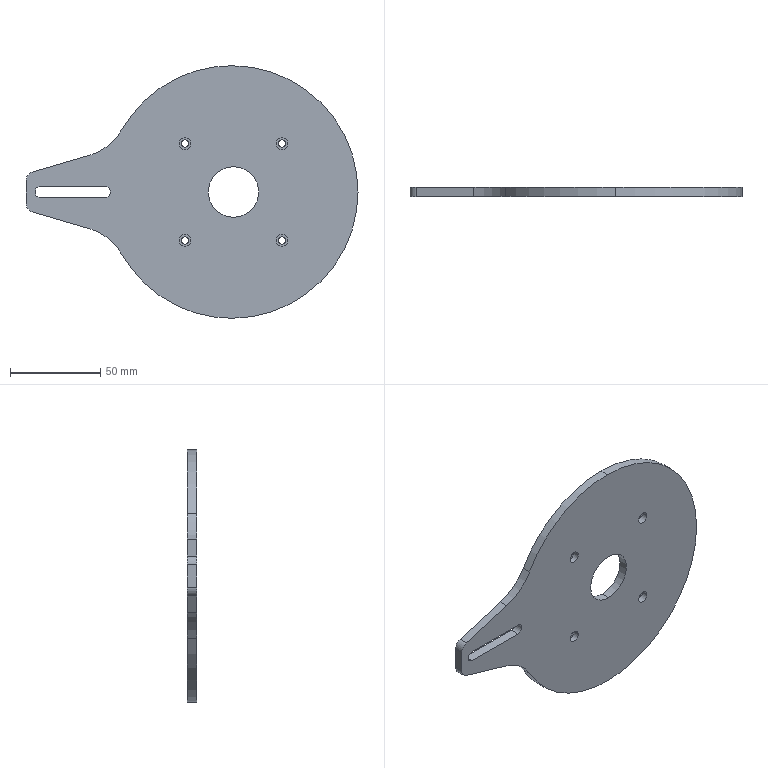Part | NX | 1 solid | 40 faces | box 184 x 5 x 140 mm | volume 79893 mm3 | cylinder 29 | plane 11 | commonest cylinder face diameters 4 x8 6.5 x8 140 x5 6 x2 10 x2 28 x2
STEP:
#1=CARTESIAN_POINT('',(-79.598,2.75,20.412));
#2=VERTEX_POINT('',#1);
#3=CARTESIAN_POINT('',(-111.411,2.75,11.056));
#4=VERTEX_POINT('',#3);
#5=CARTESIAN_POINT('',(0.,2.75,43.824));
#6=DIRECTION('',(-0.9594,0.,-0.2822));
#7=VECTOR('',#6,1000.);
#8=LINE('',#5,#7);
#9=EDGE_CURVE('',#2,#4,#8,.T.);
#10=ORIENTED_EDGE('',*,*,#9,.F.);
#11=CARTESIAN_POINT('',(-61.944,2.75,34.435));
#12=VERTEX_POINT('',#11);
#13=CARTESIAN_POINT('',(-88.063,2.75,49.193));
#14=DIRECTION('',(0.,-1.,0.));
#15=DIRECTION('',(-1.,0.,0.));
#16=AXIS2_PLACEMENT_3D('',#13,#14,#15);
#17=CIRCLE('',#16,30.);
#18=EDGE_CURVE('',#2,#12,#17,.T.);
#19=ORIENTED_EDGE('',*,*,#18,.T.);
#20=CARTESIAN_POINT('',(-1.,2.75,70.));
#21=VERTEX_POINT('',#20);
#22=CARTESIAN_POINT('',(-1.,2.75,0.));
#23=DIRECTION('',(0.,-1.,0.));
#24=DIRECTION('',(0.,0.,-1.));
#25=AXIS2_PLACEMENT_3D('',#22,#23,#24);
#26=CIRCLE('',#25,70.);
#27=EDGE_CURVE('',#21,#12,#26,.T.);
#28=ORIENTED_EDGE('',*,*,#27,.F.);
#29=CARTESIAN_POINT('',(-1.,2.75,-70.));
#30=VERTEX_POINT('',#29);
#31=CARTESIAN_POINT('',(-1.,2.75,0.));
#32=DIRECTION('',(0.,-1.,0.));
#33=DIRECTION('',(0.,0.,-1.));
#34=AXIS2_PLACEMENT_3D('',#31,#32,#33);
#35=CIRCLE('',#34,70.);
#36=EDGE_CURVE('',#30,#21,#35,.T.);
#37=ORIENTED_EDGE('',*,*,#36,.F.);
#38=CARTESIAN_POINT('',(-61.944,2.75,-34.435));
#39=VERTEX_POINT('',#38);
#40=CARTESIAN_POINT('',(-1.,2.75,0.));
#41=DIRECTION('',(0.,-1.,0.));
#42=DIRECTION('',(0.,0.,-1.));
#43=AXIS2_PLACEMENT_3D('',#40,#41,#42);
#44=CIRCLE('',#43,70.);
#45=EDGE_CURVE('',#39,#30,#44,.T.);
#46=ORIENTED_EDGE('',*,*,#45,.F.);
#47=CARTESIAN_POINT('',(-79.598,2.75,-20.412));
#48=VERTEX_POINT('',#47);
#49=CARTESIAN_POINT('',(-88.063,2.75,-49.193));
#50=DIRECTION('',(0.,-1.,0.));
#51=DIRECTION('',(-1.,0.,0.));
#52=AXIS2_PLACEMENT_3D('',#49,#50,#51);
#53=CIRCLE('',#52,30.);
#54=EDGE_CURVE('',#39,#48,#53,.T.);
#55=ORIENTED_EDGE('',*,*,#54,.T.);
#56=CARTESIAN_POINT('',(-111.411,2.75,-11.056));
#57=VERTEX_POINT('',#56);
#58=CARTESIAN_POINT('',(0.,2.75,-43.824));
#59=DIRECTION('',(0.9594,0.,-0.2822));
#60=VECTOR('',#59,1000.);
#61=LINE('',#58,#60);
#62=EDGE_CURVE('',#57,#48,#61,.T.);
#63=ORIENTED_EDGE('',*,*,#62,.F.);
#64=CARTESIAN_POINT('',(-115.,2.75,-6.259));
#65=VERTEX_POINT('',#64);
#66=CARTESIAN_POINT('',(-110.,2.75,-6.259));
#67=DIRECTION('',(0.,-1.,0.));
#68=DIRECTION('',(-1.,0.,0.));
#69=AXIS2_PLACEMENT_3D('',#66,#67,#68);
#70=CIRCLE('',#69,5.);
#71=EDGE_CURVE('',#65,#57,#70,.T.);
#72=ORIENTED_EDGE('',*,*,#71,.F.);
#73=CARTESIAN_POINT('',(-115.,2.75,6.259));
#74=VERTEX_POINT('',#73);
#75=CARTESIAN_POINT('',(-115.,2.75,0.));
#76=DIRECTION('',(0.,0.,-1.));
#77=VECTOR('',#76,1000.);
#78=LINE('',#75,#77);
#79=EDGE_CURVE('',#74,#65,#78,.T.);
#80=ORIENTED_EDGE('',*,*,#79,.F.);
#81=CARTESIAN_POINT('',(-110.,2.75,6.259));
#82=DIRECTION('',(0.,1.,0.));
#83=DIRECTION('',(1.,0.,0.));
#84=AXIS2_PLACEMENT_3D('',#81,#82,#83);
#85=CIRCLE('',#84,5.);
#86=EDGE_CURVE('',#74,#4,#85,.T.);
#87=ORIENTED_EDGE('',*,*,#86,.T.);
#88=EDGE_LOOP('',(#10,#19,#28,#37,#46,#55,#63,#72,#80,#87));
#89=FACE_BOUND('',#88,.T.);
#90=CARTESIAN_POINT('',(-28.87,2.75,26.87));
#91=VERTEX_POINT('',#90);
#92=CARTESIAN_POINT('',(-24.87,2.75,26.87));
#93=VERTEX_POINT('',#92);
#94=CARTESIAN_POINT('',(-26.87,2.75,26.87));
#95=DIRECTION('',(0.,-1.,0.));
#96=DIRECTION('',(-1.,0.,0.));
#97=AXIS2_PLACEMENT_3D('',#94,#95,#96);
#98=CIRCLE('',#97,2.);
#99=EDGE_CURVE('',#91,#93,#98,.T.);
#100=ORIENTED_EDGE('',*,*,#99,.T.);
#101=CARTESIAN_POINT('',(-26.87,2.75,26.87));
#102=DIRECTION('',(0.,-1.,0.));
#103=DIRECTION('',(-1.,0.,0.));
#104=AXIS2_PLACEMENT_3D('',#101,#102,#103);
#105=CIRCLE('',#104,2.);
#106=EDGE_CURVE('',#93,#91,#105,.T.);
#107=ORIENTED_EDGE('',*,*,#106,.T.);
#108=EDGE_LOOP('',(#100,#107));
#109=FACE_BOUND('',#108,.T.);
#110=CARTESIAN_POINT('',(-70.936,2.75,3.));
#111=VERTEX_POINT('',#110);
#112=CARTESIAN_POINT('',(-107.,2.75,3.));
#113=VERTEX_POINT('',#112);
#114=CARTESIAN_POINT('',(0.,2.75,3.));
#115=DIRECTION('',(-1.,0.,0.));
#116=VECTOR('',#115,1000.);
#117=LINE('',#114,#116);
#118=EDGE_CURVE('',#111,#113,#117,.T.);
#119=ORIENTED_EDGE('',*,*,#118,.T.);
#120=CARTESIAN_POINT('',(-107.,2.75,-3.));
#121=VERTEX_POINT('',#120);
#122=CARTESIAN_POINT('',(-107.,2.75,0.));
#123=DIRECTION('',(0.,-1.,0.));
#124=DIRECTION('',(0.,0.,-1.));
#125=AXIS2_PLACEMENT_3D('',#122,#123,#124);
#126=CIRCLE('',#125,3.);
#127=EDGE_CURVE('',#113,#121,#126,.T.);
#128=ORIENTED_EDGE('',*,*,#127,.T.);
#129=CARTESIAN_POINT('',(-70.936,2.75,-3.));
#130=VERTEX_POINT('',#129);
#131=CARTESIAN_POINT('',(0.,2.75,-3.));
#132=DIRECTION('',(1.,0.,0.));
#133=VECTOR('',#132,1000.);
#134=LINE('',#131,#133);
#135=EDGE_CURVE('',#121,#130,#134,.T.);
#136=ORIENTED_EDGE('',*,*,#135,.T.);
#137=CARTESIAN_POINT('',(-70.936,2.75,-2.988));
#138=VERTEX_POINT('',#137);
#139=CARTESIAN_POINT('',(-1.,2.75,0.));
#140=DIRECTION('',(0.,-1.,0.));
#141=DIRECTION('',(0.,0.,-1.));
#142=AXIS2_PLACEMENT_3D('',#139,#140,#141);
#143=CIRCLE('',#142,70.);
#144=EDGE_CURVE('',#138,#130,#143,.T.);
#145=ORIENTED_EDGE('',*,*,#144,.F.);
#146=CARTESIAN_POINT('',(-70.936,2.75,2.988));
#147=VERTEX_POINT('',#146);
#148=CARTESIAN_POINT('',(-71.201,2.75,0.));
#149=DIRECTION('',(0.,-1.,0.));
#150=DIRECTION('',(0.,0.,-1.));
#151=AXIS2_PLACEMENT_3D('',#148,#149,#150);
#152=CIRCLE('',#151,3.);
#153=EDGE_CURVE('',#138,#147,#152,.T.);
#154=ORIENTED_EDGE('',*,*,#153,.T.);
#155=CARTESIAN_POINT('',(-1.,2.75,0.));
#156=DIRECTION('',(0.,-1.,0.));
#157=DIRECTION('',(0.,0.,-1.));
#158=AXIS2_PLACEMENT_3D('',#155,#156,#157);
#159=CIRCLE('',#158,70.);
#160=EDGE_CURVE('',#111,#147,#159,.T.);
#161=ORIENTED_EDGE('',*,*,#160,.F.);
#162=EDGE_LOOP('',(#119,#128,#136,#145,#154,#161));
#163=FACE_BOUND('',#162,.T.);
#164=CARTESIAN_POINT('',(0.,2.75,14.));
#165=VERTEX_POINT('',#164);
#166=CARTESIAN_POINT('',(0.,2.75,-14.));
#167=VERTEX_POINT('',#166);
#168=CARTESIAN_POINT('',(0.,2.75,0.));
#169=DIRECTION('',(0.,-1.,0.));
#170=DIRECTION('',(0.,0.,-1.));
#171=AXIS2_PLACEMENT_3D('',#168,#169,#170);
#172=CIRCLE('',#171,14.);
#173=EDGE_CURVE('',#165,#167,#172,.T.);
#174=ORIENTED_EDGE('',*,*,#173,.T.);
#175=CARTESIAN_POINT('',(0.,2.75,0.));
#176=DIRECTION('',(0.,-1.,0.));
#177=DIRECTION('',(0.,0.,-1.));
#178=AXIS2_PLACEMENT_3D('',#175,#176,#177);
#179=CIRCLE('',#178,14.);
#180=EDGE_CURVE('',#167,#165,#179,.T.);
#181=ORIENTED_EDGE('',*,*,#180,.T.);
#182=EDGE_LOOP('',(#174,#181));
#183=FACE_BOUND('',#182,.T.);
#184=CARTESIAN_POINT('',(24.87,2.75,26.87));
#185=VERTEX_POINT('',#184);
#186=CARTESIAN_POINT('',(28.87,2.75,26.87));
#187=VERTEX_POINT('',#186);
#188=CARTESIAN_POINT('',(26.87,2.75,26.87));
#189=DIRECTION('',(0.,-1.,0.));
#190=DIRECTION('',(-1.,0.,0.));
#191=AXIS2_PLACEMENT_3D('',#188,#189,#190);
#192=CIRCLE('',#191,2.);
#193=EDGE_CURVE('',#185,#187,#192,.T.);
#194=ORIENTED_EDGE('',*,*,#193,.T.);
#195=CARTESIAN_POINT('',(26.87,2.75,26.87));
#196=DIRECTION('',(0.,-1.,0.));
#197=DIRECTION('',(-1.,0.,0.));
#198=AXIS2_PLACEMENT_3D('',#195,#196,#197);
#199=CIRCLE('',#198,2.);
#200=EDGE_CURVE('',#187,#185,#199,.T.);
#201=ORIENTED_EDGE('',*,*,#200,.T.);
#202=EDGE_LOOP('',(#194,#201));
#203=FACE_BOUND('',#202,.T.);
#204=CARTESIAN_POINT('',(-28.87,2.75,-26.87));
#205=VERTEX_POINT('',#204);
#206=CARTESIAN_POINT('',(-24.87,2.75,-26.87));
#207=VERTEX_POINT('',#206);
#208=CARTESIAN_POINT('',(-26.87,2.75,-26.87));
#209=DIRECTION('',(0.,-1.,0.));
#210=DIRECTION('',(-1.,0.,0.));
#211=AXIS2_PLACEMENT_3D('',#208,#209,#210);
#212=CIRCLE('',#211,2.);
#213=EDGE_CURVE('',#205,#207,#212,.T.);
#214=ORIENTED_EDGE('',*,*,#213,.T.);
#215=CARTESIAN_POINT('',(-26.87,2.75,-26.87));
#216=DIRECTION('',(0.,-1.,0.));
#217=DIRECTION('',(-1.,0.,0.));
#218=AXIS2_PLACEMENT_3D('',#215,#216,#217);
#219=CIRCLE('',#218,2.);
#220=EDGE_CURVE('',#207,#205,#219,.T.);
#221=ORIENTED_EDGE('',*,*,#220,.T.);
#222=EDGE_LOOP('',(#214,#221));
#223=FACE_BOUND('',#222,.T.);
#224=CARTESIAN_POINT('',(28.87,2.75,-26.87));
#225=VERTEX_POINT('',#224);
#226=CARTESIAN_POINT('',(24.87,2.75,-26.87));
#227=VERTEX_POINT('',#226);
#228=CARTESIAN_POINT('',(26.87,2.75,-26.87));
#229=DIRECTION('',(0.,-1.,0.));
#230=DIRECTION('',(-1.,0.,0.));
#231=AXIS2_PLACEMENT_3D('',#228,#229,#230);
#232=CIRCLE('',#231,2.);
#233=EDGE_CURVE('',#225,#227,#232,.T.);
#234=ORIENTED_EDGE('',*,*,#233,.T.);
#235=CARTESIAN_POINT('',(26.87,2.75,-26.87));
#236=DIRECTION('',(0.,-1.,0.));
#237=DIRECTION('',(-1.,0.,0.));
#238=AXIS2_PLACEMENT_3D('',#235,#236,#237);
#239=CIRCLE('',#238,2.);
#240=EDGE_CURVE('',#227,#225,#239,.T.);
#241=ORIENTED_EDGE('',*,*,#240,.T.);
#242=EDGE_LOOP('',(#234,#241));
#243=FACE_BOUND('',#242,.T.);
#244=CARTESIAN_POINT('',(0.,2.75,0.));
#245=DIRECTION('',(0.,1.,0.));
#246=DIRECTION('',(1.,0.,0.));
#247=AXIS2_PLACEMENT_3D('',#244,#245,#246);
#248=PLANE('',#247);
#249=ADVANCED_FACE('',(#89,#109,#163,#183,#203,#223,#243),#248,.T.);
#250=CARTESIAN_POINT('',(-115.,-2.25,-6.259));
#251=VERTEX_POINT('',#250);
#252=CARTESIAN_POINT('',(-115.,0.,-6.259));
#253=DIRECTION('',(0.,-1.,0.));
#254=VECTOR('',#253,1000.);
#255=LINE('',#252,#254);
#256=EDGE_CURVE('',#65,#251,#255,.T.);
#257=ORIENTED_EDGE('',*,*,#256,.T.);
#258=CARTESIAN_POINT('',(-115.,-2.25,6.259));
#259=VERTEX_POINT('',#258);
#260=CARTESIAN_POINT('',(-115.,-2.25,0.));
#261=DIRECTION('',(0.,0.,1.));
#262=VECTOR('',#261,1000.);
#263=LINE('',#260,#262);
#264=EDGE_CURVE('',#251,#259,#263,.T.);
#265=ORIENTED_EDGE('',*,*,#264,.T.);
#266=CARTESIAN_POINT('',(-115.,0.,6.259));
#267=DIRECTION('',(0.,1.,0.));
#268=VECTOR('',#267,1000.);
#269=LINE('',#266,#268);
#270=EDGE_CURVE('',#259,#74,#269,.T.);
#271=ORIENTED_EDGE('',*,*,#270,.T.);
#272=ORIENTED_EDGE('',*,*,#79,.T.);
#273=EDGE_LOOP('',(#257,#265,#271,#272));
#274=FACE_BOUND('',#273,.T.);
#275=CARTESIAN_POINT('',(-115.,-2.25,-10.));
#276=DIRECTION('',(-1.,0.,0.));
#277=DIRECTION('',(0.,0.,1.));
#278=AXIS2_PLACEMENT_3D('',#275,#276,#277);
#279=PLANE('',#278);
#280=ADVANCED_FACE('',(#274),#279,.T.);
#281=CARTESIAN_POINT('',(-70.936,-2.25,2.988));
#282=VERTEX_POINT('',#281);
#283=CARTESIAN_POINT('',(-70.936,-2.25,2.988));
#284=DIRECTION('',(0.,-1.,0.));
#285=VECTOR('',#284,1000.);
#286=LINE('',#283,#285);
#287=EDGE_CURVE('',#147,#282,#286,.T.);
#288=ORIENTED_EDGE('',*,*,#287,.T.);
#289=CARTESIAN_POINT('',(-70.936,-2.25,3.));
#290=VERTEX_POINT('',#289);
#291=CARTESIAN_POINT('',(-1.,-2.25,0.));
#292=DIRECTION('',(0.,-1.,0.));
#293=DIRECTION('',(0.,0.,-1.));
#294=AXIS2_PLACEMENT_3D('',#291,#292,#293);
#295=CIRCLE('',#294,70.);
#296=EDGE_CURVE('',#290,#282,#295,.T.);
#297=ORIENTED_EDGE('',*,*,#296,.F.);
#298=CARTESIAN_POINT('',(-70.936,-2.25,3.));
#299=DIRECTION('',(0.,-1.,0.));
#300=VECTOR('',#299,1000.);
#301=LINE('',#298,#300);
#302=EDGE_CURVE('',#111,#290,#301,.T.);
#303=ORIENTED_EDGE('',*,*,#302,.F.);
#304=ORIENTED_EDGE('',*,*,#160,.T.);
#305=EDGE_LOOP('',(#288,#297,#303,#304));
#306=FACE_BOUND('',#305,.T.);
#307=CARTESIAN_POINT('',(-1.,-2.25,0.));
#308=DIRECTION('',(0.,-1.,0.));
#309=DIRECTION('',(0.,0.,-1.));
#310=AXIS2_PLACEMENT_3D('',#307,#308,#309);
#311=CYLINDRICAL_SURFACE('',#310,70.);
#312=ADVANCED_FACE('',(#306),#311,.T.);
#313=ORIENTED_EDGE('',*,*,#144,.T.);
#314=CARTESIAN_POINT('',(-70.936,-2.25,-3.));
#315=VERTEX_POINT('',#314);
#316=CARTESIAN_POINT('',(-70.936,-2.25,-3.));
#317=DIRECTION('',(0.,-1.,0.));
#318=VECTOR('',#317,1000.);
#319=LINE('',#316,#318);
#320=EDGE_CURVE('',#130,#315,#319,.T.);
#321=ORIENTED_EDGE('',*,*,#320,.T.);
#322=CARTESIAN_POINT('',(-70.936,-2.25,-2.988));
#323=VERTEX_POINT('',#322);
#324=CARTESIAN_POINT('',(-1.,-2.25,0.));
#325=DIRECTION('',(0.,-1.,0.));
#326=DIRECTION('',(0.,0.,-1.));
#327=AXIS2_PLACEMENT_3D('',#324,#325,#326);
#328=CIRCLE('',#327,70.);
#329=EDGE_CURVE('',#323,#315,#328,.T.);
#330=ORIENTED_EDGE('',*,*,#329,.F.);
#331=CARTESIAN_POINT('',(-70.936,-2.25,-2.988));
#332=DIRECTION('',(0.,-1.,0.));
#333=VECTOR('',#332,1000.);
#334=LINE('',#331,#333);
#335=EDGE_CURVE('',#138,#323,#334,.T.);
#336=ORIENTED_EDGE('',*,*,#335,.F.);
#337=EDGE_LOOP('',(#313,#321,#330,#336));
#338=FACE_BOUND('',#337,.T.);
#339=CARTESIAN_POINT('',(-1.,-2.25,0.));
#340=DIRECTION('',(0.,-1.,0.));
#341=DIRECTION('',(0.,0.,-1.));
#342=AXIS2_PLACEMENT_3D('',#339,#340,#341);
#343=CYLINDRICAL_SURFACE('',#342,70.);
#344=ADVANCED_FACE('',(#338),#343,.T.);
#345=CARTESIAN_POINT('',(-79.598,-2.25,-20.412));
#346=VERTEX_POINT('',#345);
#347=CARTESIAN_POINT('',(-79.598,-2.25,-20.412));
#348=DIRECTION('',(0.,-1.,0.));
#349=VECTOR('',#348,1000.);
#350=LINE('',#347,#349);
#351=EDGE_CURVE('',#48,#346,#350,.T.);
#352=ORIENTED_EDGE('',*,*,#351,.T.);
#353=CARTESIAN_POINT('',(-111.411,-2.25,-11.056));
#354=VERTEX_POINT('',#353);
#355=CARTESIAN_POINT('',(0.,-2.25,-43.824));
#356=DIRECTION('',(0.9594,0.,-0.2822));
#357=VECTOR('',#356,1000.);
#358=LINE('',#355,#357);
#359=EDGE_CURVE('',#354,#346,#358,.T.);
#360=ORIENTED_EDGE('',*,*,#359,.F.);
#361=CARTESIAN_POINT('',(-111.411,0.,-11.056));
#362=DIRECTION('',(0.,-1.,0.));
#363=VECTOR('',#362,1000.);
#364=LINE('',#361,#363);
#365=EDGE_CURVE('',#57,#354,#364,.T.);
#366=ORIENTED_EDGE('',*,*,#365,.F.);
#367=ORIENTED_EDGE('',*,*,#62,.T.);
#368=EDGE_LOOP('',(#352,#360,#366,#367));
#369=FACE_BOUND('',#368,.T.);
#370=CARTESIAN_POINT('',(-30.,-2.25,-35.));
#371=DIRECTION('',(-0.2822,0.,-0.9594));
#372=DIRECTION('',(-0.9594,0.,0.2822));
#373=AXIS2_PLACEMENT_3D('',#370,#371,#372);
#374=PLANE('',#373);
#375=ADVANCED_FACE('',(#369),#374,.T.);
#376=CARTESIAN_POINT('',(-107.,-2.25,3.));
#377=VERTEX_POINT('',#376);
#378=CARTESIAN_POINT('',(-107.,-2.25,-3.));
#379=VERTEX_POINT('',#378);
#380=CARTESIAN_POINT('',(-107.,-2.25,0.));
#381=DIRECTION('',(0.,-1.,0.));
#382=DIRECTION('',(0.,0.,-1.));
#383=AXIS2_PLACEMENT_3D('',#380,#381,#382);
#384=CIRCLE('',#383,3.);
#385=EDGE_CURVE('',#377,#379,#384,.T.);
#386=ORIENTED_EDGE('',*,*,#385,.T.);
#387=CARTESIAN_POINT('',(-107.,3.25,-3.));
#388=DIRECTION('',(0.,-1.,0.));
#389=VECTOR('',#388,1000.);
#390=LINE('',#387,#389);
#391=EDGE_CURVE('',#121,#379,#390,.T.);
#392=ORIENTED_EDGE('',*,*,#391,.F.);
#393=ORIENTED_EDGE('',*,*,#127,.F.);
#394=CARTESIAN_POINT('',(-107.,-2.25,3.));
#395=DIRECTION('',(0.,1.,0.));
#396=VECTOR('',#395,1000.);
#397=LINE('',#394,#396);
#398=EDGE_CURVE('',#377,#113,#397,.T.);
#399=ORIENTED_EDGE('',*,*,#398,.F.);
#400=EDGE_LOOP('',(#386,#392,#393,#399));
#401=FACE_BOUND('',#400,.T.);
#402=CARTESIAN_POINT('',(-107.,2.25,0.));
#403=DIRECTION('',(0.,1.,0.));
#404=DIRECTION('',(1.,0.,0.));
#405=AXIS2_PLACEMENT_3D('',#402,#403,#404);
#406=CYLINDRICAL_SURFACE('',#405,3.);
#407=ADVANCED_FACE('',(#401),#406,.F.);
#408=CARTESIAN_POINT('',(-79.598,-2.25,20.412));
#409=VERTEX_POINT('',#408);
#410=CARTESIAN_POINT('',(-79.598,-2.25,20.412));
#411=DIRECTION('',(0.,-1.,0.));
#412=VECTOR('',#411,1000.);
#413=LINE('',#410,#412);
#414=EDGE_CURVE('',#2,#409,#413,.T.);
#415=ORIENTED_EDGE('',*,*,#414,.F.);
#416=ORIENTED_EDGE('',*,*,#9,.T.);
#417=CARTESIAN_POINT('',(-111.411,-2.25,11.056));
#418=VERTEX_POINT('',#417);
#419=CARTESIAN_POINT('',(-111.411,0.,11.056));
#420=DIRECTION('',(0.,1.,0.));
#421=VECTOR('',#420,1000.);
#422=LINE('',#419,#421);
#423=EDGE_CURVE('',#418,#4,#422,.T.);
#424=ORIENTED_EDGE('',*,*,#423,.F.);
#425=CARTESIAN_POINT('',(0.,-2.25,43.824));
#426=DIRECTION('',(0.9594,0.,0.2822));
#427=VECTOR('',#426,1000.);
#428=LINE('',#425,#427);
#429=EDGE_CURVE('',#418,#409,#428,.T.);
#430=ORIENTED_EDGE('',*,*,#429,.T.);
#431=EDGE_LOOP('',(#415,#416,#424,#430));
#432=FACE_BOUND('',#431,.T.);
#433=CARTESIAN_POINT('',(-115.,-2.25,10.));
#434=DIRECTION('',(-0.2822,0.,0.9594));
#435=DIRECTION('',(0.,1.,0.));
#436=AXIS2_PLACEMENT_3D('',#433,#434,#435);
#437=PLANE('',#436);
#438=ADVANCED_FACE('',(#432),#437,.T.);
#439=CARTESIAN_POINT('',(-1.,-2.25,70.));
#440=VERTEX_POINT('',#439);
#441=CARTESIAN_POINT('',(-1.,-2.25,70.));
#442=DIRECTION('',(0.,-1.,0.));
#443=VECTOR('',#442,1000.);
#444=LINE('',#441,#443);
#445=EDGE_CURVE('',#21,#440,#444,.T.);
#446=ORIENTED_EDGE('',*,*,#445,.F.);
#447=ORIENTED_EDGE('',*,*,#27,.T.);
#448=CARTESIAN_POINT('',(-61.944,-2.25,34.435));
#449=VERTEX_POINT('',#448);
#450=CARTESIAN_POINT('',(-61.944,-2.25,34.435));
#451=DIRECTION('',(0.,-1.,0.));
#452=VECTOR('',#451,1000.);
#453=LINE('',#450,#452);
#454=EDGE_CURVE('',#12,#449,#453,.T.);
#455=ORIENTED_EDGE('',*,*,#454,.T.);
#456=CARTESIAN_POINT('',(-1.,-2.25,0.));
#457=DIRECTION('',(0.,-1.,0.));
#458=DIRECTION('',(0.,0.,-1.));
#459=AXIS2_PLACEMENT_3D('',#456,#457,#458);
#460=CIRCLE('',#459,70.);
#461=EDGE_CURVE('',#440,#449,#460,.T.);
#462=ORIENTED_EDGE('',*,*,#461,.F.);
#463=EDGE_LOOP('',(#446,#447,#455,#462));
#464=FACE_BOUND('',#463,.T.);
#465=CARTESIAN_POINT('',(-1.,-2.25,0.));
#466=DIRECTION('',(0.,-1.,0.));
#467=DIRECTION('',(0.,0.,-1.));
#468=AXIS2_PLACEMENT_3D('',#465,#466,#467);
#469=CYLINDRICAL_SURFACE('',#468,70.);
#470=ADVANCED_FACE('',(#464),#469,.T.);
#471=ORIENTED_EDGE('',*,*,#335,.T.);
#472=CARTESIAN_POINT('',(-71.201,-2.25,0.));
#473=DIRECTION('',(0.,-1.,0.));
#474=DIRECTION('',(0.,0.,-1.));
#475=AXIS2_PLACEMENT_3D('',#472,#473,#474);
#476=CIRCLE('',#475,3.);
#477=EDGE_CURVE('',#323,#282,#476,.T.);
#478=ORIENTED_EDGE('',*,*,#477,.T.);
#479=ORIENTED_EDGE('',*,*,#287,.F.);
#480=ORIENTED_EDGE('',*,*,#153,.F.);
#481=EDGE_LOOP('',(#471,#478,#479,#480));
#482=FACE_BOUND('',#481,.T.);
#483=CARTESIAN_POINT('',(-71.201,3.25,0.));
#484=DIRECTION('',(0.,-1.,0.));
#485=DIRECTION('',(0.,0.,-1.));
#486=AXIS2_PLACEMENT_3D('',#483,#484,#485);
#487=CYLINDRICAL_SURFACE('',#486,3.);
#488=ADVANCED_FACE('',(#482),#487,.F.);
#489=ORIENTED_EDGE('',*,*,#429,.F.);
#490=CARTESIAN_POINT('',(-110.,-2.25,6.259));
#491=DIRECTION('',(0.,1.,0.));
#492=DIRECTION('',(1.,0.,0.));
#493=AXIS2_PLACEMENT_3D('',#490,#491,#492);
#494=CIRCLE('',#493,5.);
#495=EDGE_CURVE('',#259,#418,#494,.T.);
#496=ORIENTED_EDGE('',*,*,#495,.F.);
#497=ORIENTED_EDGE('',*,*,#264,.F.);
#498=CARTESIAN_POINT('',(-110.,-2.25,-6.259));
#499=DIRECTION('',(0.,-1.,0.));
#500=DIRECTION('',(-1.,0.,0.));
#501=AXIS2_PLACEMENT_3D('',#498,#499,#500);
#502=CIRCLE('',#501,5.);
#503=EDGE_CURVE('',#251,#354,#502,.T.);
#504=ORIENTED_EDGE('',*,*,#503,.T.);
#505=ORIENTED_EDGE('',*,*,#359,.T.);
#506=CARTESIAN_POINT('',(-61.944,-2.25,-34.435));
#507=VERTEX_POINT('',#506);
#508=CARTESIAN_POINT('',(-88.063,-2.25,-49.193));
#509=DIRECTION('',(0.,-1.,0.));
#510=DIRECTION('',(-1.,0.,0.));
#511=AXIS2_PLACEMENT_3D('',#508,#509,#510);
#512=CIRCLE('',#511,30.);
#513=EDGE_CURVE('',#507,#346,#512,.T.);
#514=ORIENTED_EDGE('',*,*,#513,.F.);
#515=CARTESIAN_POINT('',(-1.,-2.25,-70.));
#516=VERTEX_POINT('',#515);
#517=CARTESIAN_POINT('',(-1.,-2.25,0.));
#518=DIRECTION('',(0.,-1.,0.));
#519=DIRECTION('',(0.,0.,-1.));
#520=AXIS2_PLACEMENT_3D('',#517,#518,#519);
#521=CIRCLE('',#520,70.);
#522=EDGE_CURVE('',#507,#516,#521,.T.);
#523=ORIENTED_EDGE('',*,*,#522,.T.);
#524=CARTESIAN_POINT('',(-1.,-2.25,0.));
#525=DIRECTION('',(0.,-1.,0.));
#526=DIRECTION('',(0.,0.,-1.));
#527=AXIS2_PLACEMENT_3D('',#524,#525,#526);
#528=CIRCLE('',#527,70.);
#529=EDGE_CURVE('',#516,#440,#528,.T.);
#530=ORIENTED_EDGE('',*,*,#529,.T.);
#531=ORIENTED_EDGE('',*,*,#461,.T.);
#532=CARTESIAN_POINT('',(-88.063,-2.25,49.193));
#533=DIRECTION('',(0.,-1.,0.));
#534=DIRECTION('',(-1.,0.,0.));
#535=AXIS2_PLACEMENT_3D('',#532,#533,#534);
#536=CIRCLE('',#535,30.);
#537=EDGE_CURVE('',#409,#449,#536,.T.);
#538=ORIENTED_EDGE('',*,*,#537,.F.);
#539=EDGE_LOOP('',(#489,#496,#497,#504,#505,#514,#523,#530,#531,#538));
#540=FACE_BOUND('',#539,.T.);
#541=CARTESIAN_POINT('',(0.,-2.25,3.));
#542=DIRECTION('',(-1.,0.,0.));
#543=VECTOR('',#542,1000.);
#544=LINE('',#541,#543);
#545=EDGE_CURVE('',#290,#377,#544,.T.);
#546=ORIENTED_EDGE('',*,*,#545,.F.);
#547=ORIENTED_EDGE('',*,*,#296,.T.);
#548=ORIENTED_EDGE('',*,*,#477,.F.);
#549=ORIENTED_EDGE('',*,*,#329,.T.);
#550=CARTESIAN_POINT('',(0.,-2.25,-3.));
#551=DIRECTION('',(1.,0.,0.));
#552=VECTOR('',#551,1000.);
#553=LINE('',#550,#552);
#554=EDGE_CURVE('',#379,#315,#553,.T.);
#555=ORIENTED_EDGE('',*,*,#554,.F.);
#556=ORIENTED_EDGE('',*,*,#385,.F.);
#557=EDGE_LOOP('',(#546,#547,#548,#549,#555,#556));
#558=FACE_BOUND('',#557,.T.);
#559=CARTESIAN_POINT('',(0.,-2.25,14.));
#560=VERTEX_POINT('',#559);
#561=CARTESIAN_POINT('',(0.,-2.25,-14.));
#562=VERTEX_POINT('',#561);
#563=CARTESIAN_POINT('',(0.,-2.25,0.));
#564=DIRECTION('',(0.,-1.,0.));
#565=DIRECTION('',(0.,0.,-1.));
#566=AXIS2_PLACEMENT_3D('',#563,#564,#565);
#567=CIRCLE('',#566,14.);
#568=EDGE_CURVE('',#560,#562,#567,.T.);
#569=ORIENTED_EDGE('',*,*,#568,.F.);
#570=CARTESIAN_POINT('',(0.,-2.25,0.));
#571=DIRECTION('',(0.,-1.,0.));
#572=DIRECTION('',(0.,0.,-1.));
#573=AXIS2_PLACEMENT_3D('',#570,#571,#572);
#574=CIRCLE('',#573,14.);
#575=EDGE_CURVE('',#562,#560,#574,.T.);
#576=ORIENTED_EDGE('',*,*,#575,.F.);
#577=EDGE_LOOP('',(#569,#576));
#578=FACE_BOUND('',#577,.T.);
#579=CARTESIAN_POINT('',(-23.62,-2.25,26.87));
#580=VERTEX_POINT('',#579);
#581=CARTESIAN_POINT('',(-30.12,-2.25,26.87));
#582=VERTEX_POINT('',#581);
#583=CARTESIAN_POINT('',(-26.87,-2.25,26.87));
#584=DIRECTION('',(0.,-1.,0.));
#585=DIRECTION('',(-1.,0.,0.));
#586=AXIS2_PLACEMENT_3D('',#583,#584,#585);
#587=CIRCLE('',#586,3.25);
#588=EDGE_CURVE('',#580,#582,#587,.T.);
#589=ORIENTED_EDGE('',*,*,#588,.F.);
#590=CARTESIAN_POINT('',(-26.87,-2.25,26.87));
#591=DIRECTION('',(0.,-1.,0.));
#592=DIRECTION('',(-1.,0.,0.));
#593=AXIS2_PLACEMENT_3D('',#590,#591,#592);
#594=CIRCLE('',#593,3.25);
#595=EDGE_CURVE('',#582,#580,#594,.T.);
#596=ORIENTED_EDGE('',*,*,#595,.F.);
#597=EDGE_LOOP('',(#589,#596));
#598=FACE_BOUND('',#597,.T.);
#599=CARTESIAN_POINT('',(30.12,-2.25,-26.87));
#600=VERTEX_POINT('',#599);
#601=CARTESIAN_POINT('',(23.62,-2.25,-26.87));
#602=VERTEX_POINT('',#601);
#603=CARTESIAN_POINT('',(26.87,-2.25,-26.87));
#604=DIRECTION('',(0.,-1.,0.));
#605=DIRECTION('',(-1.,0.,0.));
#606=AXIS2_PLACEMENT_3D('',#603,#604,#605);
#607=CIRCLE('',#606,3.25);
#608=EDGE_CURVE('',#600,#602,#607,.T.);
#609=ORIENTED_EDGE('',*,*,#608,.F.);
#610=CARTESIAN_POINT('',(26.87,-2.25,-26.87));
#611=DIRECTION('',(0.,-1.,0.));
#612=DIRECTION('',(-1.,0.,0.));
#613=AXIS2_PLACEMENT_3D('',#610,#611,#612);
#614=CIRCLE('',#613,3.25);
#615=EDGE_CURVE('',#602,#600,#614,.T.);
#616=ORIENTED_EDGE('',*,*,#615,.F.);
#617=EDGE_LOOP('',(#609,#616));
#618=FACE_BOUND('',#617,.T.);
#619=CARTESIAN_POINT('',(-30.12,-2.25,-26.87));
#620=VERTEX_POINT('',#619);
#621=CARTESIAN_POINT('',(-23.62,-2.25,-26.87));
#622=VERTEX_POINT('',#621);
#623=CARTESIAN_POINT('',(-26.87,-2.25,-26.87));
#624=DIRECTION('',(0.,-1.,0.));
#625=DIRECTION('',(-1.,0.,0.));
#626=AXIS2_PLACEMENT_3D('',#623,#624,#625);
#627=CIRCLE('',#626,3.25);
#628=EDGE_CURVE('',#620,#622,#627,.T.);
#629=ORIENTED_EDGE('',*,*,#628,.F.);
#630=CARTESIAN_POINT('',(-26.87,-2.25,-26.87));
#631=DIRECTION('',(0.,-1.,0.));
#632=DIRECTION('',(-1.,0.,0.));
#633=AXIS2_PLACEMENT_3D('',#630,#631,#632);
#634=CIRCLE('',#633,3.25);
#635=EDGE_CURVE('',#622,#620,#634,.T.);
#636=ORIENTED_EDGE('',*,*,#635,.F.);
#637=EDGE_LOOP('',(#629,#636));
#638=FACE_BOUND('',#637,.T.);
#639=CARTESIAN_POINT('',(30.12,-2.25,26.87));
#640=VERTEX_POINT('',#639);
#641=CARTESIAN_POINT('',(23.62,-2.25,26.87));
#642=VERTEX_POINT('',#641);
#643=CARTESIAN_POINT('',(26.87,-2.25,26.87));
#644=DIRECTION('',(0.,-1.,0.));
#645=DIRECTION('',(-1.,0.,0.));
#646=AXIS2_PLACEMENT_3D('',#643,#644,#645);
#647=CIRCLE('',#646,3.25);
#648=EDGE_CURVE('',#640,#642,#647,.T.);
#649=ORIENTED_EDGE('',*,*,#648,.F.);
#650=CARTESIAN_POINT('',(26.87,-2.25,26.87));
#651=DIRECTION('',(0.,-1.,0.));
#652=DIRECTION('',(-1.,0.,0.));
#653=AXIS2_PLACEMENT_3D('',#650,#651,#652);
#654=CIRCLE('',#653,3.25);
#655=EDGE_CURVE('',#642,#640,#654,.T.);
#656=ORIENTED_EDGE('',*,*,#655,.F.);
#657=EDGE_LOOP('',(#649,#656));
#658=FACE_BOUND('',#657,.T.);
#659=CARTESIAN_POINT('',(-25.855,-2.25,-5.725));
#660=DIRECTION('',(0.,-1.,0.));
#661=DIRECTION('',(0.,0.,-1.));
#662=AXIS2_PLACEMENT_3D('',#659,#660,#661);
#663=PLANE('',#662);
#664=ADVANCED_FACE('',(#540,#558,#578,#598,#618,#638,#658),#663,.T.);
#665=ORIENTED_EDGE('',*,*,#568,.T.);
#666=CARTESIAN_POINT('',(0.,3.25,-14.));
#667=DIRECTION('',(0.,-1.,0.));
#668=VECTOR('',#667,1000.);
#669=LINE('',#666,#668);
#670=EDGE_CURVE('',#562,#167,#669,.F.);
#671=ORIENTED_EDGE('',*,*,#670,.T.);
#672=ORIENTED_EDGE('',*,*,#173,.F.);
#673=CARTESIAN_POINT('',(0.,3.25,14.));
#674=DIRECTION('',(0.,-1.,0.));
#675=VECTOR('',#674,1000.);
#676=LINE('',#673,#675);
#677=EDGE_CURVE('',#560,#165,#676,.F.);
#678=ORIENTED_EDGE('',*,*,#677,.F.);
#679=EDGE_LOOP('',(#665,#671,#672,#678));
#680=FACE_BOUND('',#679,.T.);
#681=CARTESIAN_POINT('',(0.,3.25,0.));
#682=DIRECTION('',(0.,-1.,0.));
#683=DIRECTION('',(0.,0.,-1.));
#684=AXIS2_PLACEMENT_3D('',#681,#682,#683);
#685=CYLINDRICAL_SURFACE('',#684,14.);
#686=ADVANCED_FACE('',(#680),#685,.F.);
#687=CARTESIAN_POINT('',(-23.62,1.25,26.87));
#688=VERTEX_POINT('',#687);
#689=CARTESIAN_POINT('',(-30.12,1.25,26.87));
#690=VERTEX_POINT('',#689);
#691=CARTESIAN_POINT('',(-26.87,1.25,26.87));
#692=DIRECTION('',(0.,-1.,0.));
#693=DIRECTION('',(-1.,0.,0.));
#694=AXIS2_PLACEMENT_3D('',#691,#692,#693);
#695=CIRCLE('',#694,3.25);
#696=EDGE_CURVE('',#688,#690,#695,.T.);
#697=ORIENTED_EDGE('',*,*,#696,.F.);
#698=CARTESIAN_POINT('',(-23.62,-2.25,26.87));
#699=DIRECTION('',(0.,-1.,0.));
#700=VECTOR('',#699,1000.);
#701=LINE('',#698,#700);
#702=EDGE_CURVE('',#580,#688,#701,.F.);
#703=ORIENTED_EDGE('',*,*,#702,.F.);
#704=ORIENTED_EDGE('',*,*,#588,.T.);
#705=CARTESIAN_POINT('',(-30.12,-2.25,26.87));
#706=DIRECTION('',(0.,-1.,0.));
#707=VECTOR('',#706,1000.);
#708=LINE('',#705,#707);
#709=EDGE_CURVE('',#582,#690,#708,.F.);
#710=ORIENTED_EDGE('',*,*,#709,.T.);
#711=EDGE_LOOP('',(#697,#703,#704,#710));
#712=FACE_BOUND('',#711,.T.);
#713=CARTESIAN_POINT('',(-26.87,-2.25,26.87));
#714=DIRECTION('',(0.,-1.,0.));
#715=DIRECTION('',(-1.,0.,0.));
#716=AXIS2_PLACEMENT_3D('',#713,#714,#715);
#717=CYLINDRICAL_SURFACE('',#716,3.25);
#718=ADVANCED_FACE('',(#712),#717,.F.);
#719=ORIENTED_EDGE('',*,*,#696,.T.);
#720=CARTESIAN_POINT('',(-26.87,1.25,26.87));
#721=DIRECTION('',(0.,-1.,0.));
#722=DIRECTION('',(-1.,0.,0.));
#723=AXIS2_PLACEMENT_3D('',#720,#721,#722);
#724=CIRCLE('',#723,3.25);
#725=EDGE_CURVE('',#690,#688,#724,.T.);
#726=ORIENTED_EDGE('',*,*,#725,.T.);
#727=EDGE_LOOP('',(#719,#726));
#728=FACE_BOUND('',#727,.T.);
#729=CARTESIAN_POINT('',(-24.87,1.25,26.87));
#730=VERTEX_POINT('',#729);
#731=CARTESIAN_POINT('',(-28.87,1.25,26.87));
#732=VERTEX_POINT('',#731);
#733=CARTESIAN_POINT('',(-26.87,1.25,26.87));
#734=DIRECTION('',(0.,-1.,0.));
#735=DIRECTION('',(-1.,0.,0.));
#736=AXIS2_PLACEMENT_3D('',#733,#734,#735);
#737=CIRCLE('',#736,2.);
#738=EDGE_CURVE('',#730,#732,#737,.T.);
#739=ORIENTED_EDGE('',*,*,#738,.F.);
#740=CARTESIAN_POINT('',(-26.87,1.25,26.87));
#741=DIRECTION('',(0.,-1.,0.));
#742=DIRECTION('',(-1.,0.,0.));
#743=AXIS2_PLACEMENT_3D('',#740,#741,#742);
#744=CIRCLE('',#743,2.);
#745=EDGE_CURVE('',#732,#730,#744,.T.);
#746=ORIENTED_EDGE('',*,*,#745,.F.);
#747=EDGE_LOOP('',(#739,#746));
#748=FACE_BOUND('',#747,.T.);
#749=CARTESIAN_POINT('',(-26.87,1.25,26.87));
#750=DIRECTION('',(0.,-1.,0.));
#751=DIRECTION('',(0.,0.,-1.));
#752=AXIS2_PLACEMENT_3D('',#749,#750,#751);
#753=PLANE('',#752);
#754=ADVANCED_FACE('',(#728,#748),#753,.T.);
#755=ORIENTED_EDGE('',*,*,#99,.F.);
#756=CARTESIAN_POINT('',(-28.87,-2.25,26.87));
#757=DIRECTION('',(0.,-1.,0.));
#758=VECTOR('',#757,1000.);
#759=LINE('',#756,#758);
#760=EDGE_CURVE('',#732,#91,#759,.F.);
#761=ORIENTED_EDGE('',*,*,#760,.F.);
#762=ORIENTED_EDGE('',*,*,#745,.T.);
#763=CARTESIAN_POINT('',(-24.87,-2.25,26.87));
#764=DIRECTION('',(0.,-1.,0.));
#765=VECTOR('',#764,1000.);
#766=LINE('',#763,#765);
#767=EDGE_CURVE('',#730,#93,#766,.F.);
#768=ORIENTED_EDGE('',*,*,#767,.T.);
#769=EDGE_LOOP('',(#755,#761,#762,#768));
#770=FACE_BOUND('',#769,.T.);
#771=CARTESIAN_POINT('',(-26.87,-2.25,26.87));
#772=DIRECTION('',(0.,-1.,0.));
#773=DIRECTION('',(-1.,0.,0.));
#774=AXIS2_PLACEMENT_3D('',#771,#772,#773);
#775=CYLINDRICAL_SURFACE('',#774,2.);
#776=ADVANCED_FACE('',(#770),#775,.F.);
#777=CARTESIAN_POINT('',(30.12,1.25,-26.87));
#778=VERTEX_POINT('',#777);
#779=CARTESIAN_POINT('',(23.62,1.25,-26.87));
#780=VERTEX_POINT('',#779);
#781=CARTESIAN_POINT('',(26.87,1.25,-26.87));
#782=DIRECTION('',(0.,-1.,0.));
#783=DIRECTION('',(-1.,0.,0.));
#784=AXIS2_PLACEMENT_3D('',#781,#782,#783);
#785=CIRCLE('',#784,3.25);
#786=EDGE_CURVE('',#778,#780,#785,.T.);
#787=ORIENTED_EDGE('',*,*,#786,.F.);
#788=CARTESIAN_POINT('',(30.12,-2.25,-26.87));
#789=DIRECTION('',(0.,-1.,0.));
#790=VECTOR('',#789,1000.);
#791=LINE('',#788,#790);
#792=EDGE_CURVE('',#600,#778,#791,.F.);
#793=ORIENTED_EDGE('',*,*,#792,.F.);
#794=ORIENTED_EDGE('',*,*,#608,.T.);
#795=CARTESIAN_POINT('',(23.62,-2.25,-26.87));
#796=DIRECTION('',(0.,-1.,0.));
#797=VECTOR('',#796,1000.);
#798=LINE('',#795,#797);
#799=EDGE_CURVE('',#602,#780,#798,.F.);
#800=ORIENTED_EDGE('',*,*,#799,.T.);
#801=EDGE_LOOP('',(#787,#793,#794,#800));
#802=FACE_BOUND('',#801,.T.);
#803=CARTESIAN_POINT('',(26.87,-2.25,-26.87));
#804=DIRECTION('',(0.,-1.,0.));
#805=DIRECTION('',(-1.,0.,0.));
#806=AXIS2_PLACEMENT_3D('',#803,#804,#805);
#807=CYLINDRICAL_SURFACE('',#806,3.25);
#808=ADVANCED_FACE('',(#802),#807,.F.);
#809=ORIENTED_EDGE('',*,*,#786,.T.);
#810=CARTESIAN_POINT('',(26.87,1.25,-26.87));
#811=DIRECTION('',(0.,-1.,0.));
#812=DIRECTION('',(-1.,0.,0.));
#813=AXIS2_PLACEMENT_3D('',#810,#811,#812);
#814=CIRCLE('',#813,3.25);
#815=EDGE_CURVE('',#780,#778,#814,.T.);
#816=ORIENTED_EDGE('',*,*,#815,.T.);
#817=EDGE_LOOP('',(#809,#816));
#818=FACE_BOUND('',#817,.T.);
#819=CARTESIAN_POINT('',(28.87,1.25,-26.87));
#820=VERTEX_POINT('',#819);
#821=CARTESIAN_POINT('',(24.87,1.25,-26.87));
#822=VERTEX_POINT('',#821);
#823=CARTESIAN_POINT('',(26.87,1.25,-26.87));
#824=DIRECTION('',(0.,-1.,0.));
#825=DIRECTION('',(-1.,0.,0.));
#826=AXIS2_PLACEMENT_3D('',#823,#824,#825);
#827=CIRCLE('',#826,2.);
#828=EDGE_CURVE('',#820,#822,#827,.T.);
#829=ORIENTED_EDGE('',*,*,#828,.F.);
#830=CARTESIAN_POINT('',(26.87,1.25,-26.87));
#831=DIRECTION('',(0.,-1.,0.));
#832=DIRECTION('',(-1.,0.,0.));
#833=AXIS2_PLACEMENT_3D('',#830,#831,#832);
#834=CIRCLE('',#833,2.);
#835=EDGE_CURVE('',#822,#820,#834,.T.);
#836=ORIENTED_EDGE('',*,*,#835,.F.);
#837=EDGE_LOOP('',(#829,#836));
#838=FACE_BOUND('',#837,.T.);
#839=CARTESIAN_POINT('',(26.87,1.25,-26.87));
#840=DIRECTION('',(0.,-1.,0.));
#841=DIRECTION('',(0.,0.,-1.));
#842=AXIS2_PLACEMENT_3D('',#839,#840,#841);
#843=PLANE('',#842);
#844=ADVANCED_FACE('',(#818,#838),#843,.T.);
#845=ORIENTED_EDGE('',*,*,#828,.T.);
#846=CARTESIAN_POINT('',(24.87,-2.25,-26.87));
#847=DIRECTION('',(0.,-1.,0.));
#848=VECTOR('',#847,1000.);
#849=LINE('',#846,#848);
#850=EDGE_CURVE('',#822,#227,#849,.F.);
#851=ORIENTED_EDGE('',*,*,#850,.T.);
#852=ORIENTED_EDGE('',*,*,#233,.F.);
#853=CARTESIAN_POINT('',(28.87,-2.25,-26.87));
#854=DIRECTION('',(0.,-1.,0.));
#855=VECTOR('',#854,1000.);
#856=LINE('',#853,#855);
#857=EDGE_CURVE('',#820,#225,#856,.F.);
#858=ORIENTED_EDGE('',*,*,#857,.F.);
#859=EDGE_LOOP('',(#845,#851,#852,#858));
#860=FACE_BOUND('',#859,.T.);
#861=CARTESIAN_POINT('',(26.87,-2.25,-26.87));
#862=DIRECTION('',(0.,-1.,0.));
#863=DIRECTION('',(-1.,0.,0.));
#864=AXIS2_PLACEMENT_3D('',#861,#862,#863);
#865=CYLINDRICAL_SURFACE('',#864,2.);
#866=ADVANCED_FACE('',(#860),#865,.F.);
#867=CARTESIAN_POINT('',(-23.62,1.25,-26.87));
#868=VERTEX_POINT('',#867);
#869=CARTESIAN_POINT('',(-30.12,1.25,-26.87));
#870=VERTEX_POINT('',#869);
#871=CARTESIAN_POINT('',(-26.87,1.25,-26.87));
#872=DIRECTION('',(0.,-1.,0.));
#873=DIRECTION('',(-1.,0.,0.));
#874=AXIS2_PLACEMENT_3D('',#871,#872,#873);
#875=CIRCLE('',#874,3.25);
#876=EDGE_CURVE('',#868,#870,#875,.T.);
#877=ORIENTED_EDGE('',*,*,#876,.F.);
#878=CARTESIAN_POINT('',(-23.62,-2.25,-26.87));
#879=DIRECTION('',(0.,-1.,0.));
#880=VECTOR('',#879,1000.);
#881=LINE('',#878,#880);
#882=EDGE_CURVE('',#868,#622,#881,.T.);
#883=ORIENTED_EDGE('',*,*,#882,.T.);
#884=ORIENTED_EDGE('',*,*,#635,.T.);
#885=CARTESIAN_POINT('',(-30.12,-2.25,-26.87));
#886=DIRECTION('',(0.,-1.,0.));
#887=VECTOR('',#886,1000.);
#888=LINE('',#885,#887);
#889=EDGE_CURVE('',#870,#620,#888,.T.);
#890=ORIENTED_EDGE('',*,*,#889,.F.);
#891=EDGE_LOOP('',(#877,#883,#884,#890));
#892=FACE_BOUND('',#891,.T.);
#893=CARTESIAN_POINT('',(-26.87,-2.25,-26.87));
#894=DIRECTION('',(0.,-1.,0.));
#895=DIRECTION('',(-1.,0.,0.));
#896=AXIS2_PLACEMENT_3D('',#893,#894,#895);
#897=CYLINDRICAL_SURFACE('',#896,3.25);
#898=ADVANCED_FACE('',(#892),#897,.F.);
#899=ORIENTED_EDGE('',*,*,#876,.T.);
#900=CARTESIAN_POINT('',(-26.87,1.25,-26.87));
#901=DIRECTION('',(0.,-1.,0.));
#902=DIRECTION('',(-1.,0.,0.));
#903=AXIS2_PLACEMENT_3D('',#900,#901,#902);
#904=CIRCLE('',#903,3.25);
#905=EDGE_CURVE('',#870,#868,#904,.T.);
#906=ORIENTED_EDGE('',*,*,#905,.T.);
#907=EDGE_LOOP('',(#899,#906));
#908=FACE_BOUND('',#907,.T.);
#909=CARTESIAN_POINT('',(-24.87,1.25,-26.87));
#910=VERTEX_POINT('',#909);
#911=CARTESIAN_POINT('',(-28.87,1.25,-26.87));
#912=VERTEX_POINT('',#911);
#913=CARTESIAN_POINT('',(-26.87,1.25,-26.87));
#914=DIRECTION('',(0.,-1.,0.));
#915=DIRECTION('',(-1.,0.,0.));
#916=AXIS2_PLACEMENT_3D('',#913,#914,#915);
#917=CIRCLE('',#916,2.);
#918=EDGE_CURVE('',#910,#912,#917,.T.);
#919=ORIENTED_EDGE('',*,*,#918,.F.);
#920=CARTESIAN_POINT('',(-26.87,1.25,-26.87));
#921=DIRECTION('',(0.,-1.,0.));
#922=DIRECTION('',(-1.,0.,0.));
#923=AXIS2_PLACEMENT_3D('',#920,#921,#922);
#924=CIRCLE('',#923,2.);
#925=EDGE_CURVE('',#912,#910,#924,.T.);
#926=ORIENTED_EDGE('',*,*,#925,.F.);
#927=EDGE_LOOP('',(#919,#926));
#928=FACE_BOUND('',#927,.T.);
#929=CARTESIAN_POINT('',(-26.87,1.25,-26.87));
#930=DIRECTION('',(0.,-1.,0.));
#931=DIRECTION('',(0.,0.,-1.));
#932=AXIS2_PLACEMENT_3D('',#929,#930,#931);
#933=PLANE('',#932);
#934=ADVANCED_FACE('',(#908,#928),#933,.T.);
#935=ORIENTED_EDGE('',*,*,#213,.F.);
#936=CARTESIAN_POINT('',(-28.87,-2.25,-26.87));
#937=DIRECTION('',(0.,-1.,0.));
#938=VECTOR('',#937,1000.);
#939=LINE('',#936,#938);
#940=EDGE_CURVE('',#912,#205,#939,.F.);
#941=ORIENTED_EDGE('',*,*,#940,.F.);
#942=ORIENTED_EDGE('',*,*,#925,.T.);
#943=CARTESIAN_POINT('',(-24.87,-2.25,-26.87));
#944=DIRECTION('',(0.,-1.,0.));
#945=VECTOR('',#944,1000.);
#946=LINE('',#943,#945);
#947=EDGE_CURVE('',#910,#207,#946,.F.);
#948=ORIENTED_EDGE('',*,*,#947,.T.);
#949=EDGE_LOOP('',(#935,#941,#942,#948));
#950=FACE_BOUND('',#949,.T.);
#951=CARTESIAN_POINT('',(-26.87,-2.25,-26.87));
#952=DIRECTION('',(0.,-1.,0.));
#953=DIRECTION('',(-1.,0.,0.));
#954=AXIS2_PLACEMENT_3D('',#951,#952,#953);
#955=CYLINDRICAL_SURFACE('',#954,2.);
#956=ADVANCED_FACE('',(#950),#955,.F.);
#957=CARTESIAN_POINT('',(23.62,1.25,26.87));
#958=VERTEX_POINT('',#957);
#959=CARTESIAN_POINT('',(30.12,1.25,26.87));
#960=VERTEX_POINT('',#959);
#961=CARTESIAN_POINT('',(26.87,1.25,26.87));
#962=DIRECTION('',(0.,-1.,0.));
#963=DIRECTION('',(-1.,0.,0.));
#964=AXIS2_PLACEMENT_3D('',#961,#962,#963);
#965=CIRCLE('',#964,3.25);
#966=EDGE_CURVE('',#958,#960,#965,.T.);
#967=ORIENTED_EDGE('',*,*,#966,.F.);
#968=CARTESIAN_POINT('',(23.62,-2.25,26.87));
#969=DIRECTION('',(0.,-1.,0.));
#970=VECTOR('',#969,1000.);
#971=LINE('',#968,#970);
#972=EDGE_CURVE('',#642,#958,#971,.F.);
#973=ORIENTED_EDGE('',*,*,#972,.F.);
#974=ORIENTED_EDGE('',*,*,#655,.T.);
#975=CARTESIAN_POINT('',(30.12,-2.25,26.87));
#976=DIRECTION('',(0.,-1.,0.));
#977=VECTOR('',#976,1000.);
#978=LINE('',#975,#977);
#979=EDGE_CURVE('',#640,#960,#978,.F.);
#980=ORIENTED_EDGE('',*,*,#979,.T.);
#981=EDGE_LOOP('',(#967,#973,#974,#980));
#982=FACE_BOUND('',#981,.T.);
#983=CARTESIAN_POINT('',(26.87,-2.25,26.87));
#984=DIRECTION('',(0.,-1.,0.));
#985=DIRECTION('',(-1.,0.,0.));
#986=AXIS2_PLACEMENT_3D('',#983,#984,#985);
#987=CYLINDRICAL_SURFACE('',#986,3.25);
#988=ADVANCED_FACE('',(#982),#987,.F.);
#989=ORIENTED_EDGE('',*,*,#966,.T.);
#990=CARTESIAN_POINT('',(26.87,1.25,26.87));
#991=DIRECTION('',(0.,-1.,0.));
#992=DIRECTION('',(-1.,0.,0.));
#993=AXIS2_PLACEMENT_3D('',#990,#991,#992);
#994=CIRCLE('',#993,3.25);
#995=EDGE_CURVE('',#960,#958,#994,.T.);
#996=ORIENTED_EDGE('',*,*,#995,.T.);
#997=EDGE_LOOP('',(#989,#996));
#998=FACE_BOUND('',#997,.T.);
#999=CARTESIAN_POINT('',(28.87,1.25,26.87));
#1000=VERTEX_POINT('',#999);
#1001=CARTESIAN_POINT('',(24.87,1.25,26.87));
#1002=VERTEX_POINT('',#1001);
#1003=CARTESIAN_POINT('',(26.87,1.25,26.87));
#1004=DIRECTION('',(0.,-1.,0.));
#1005=DIRECTION('',(-1.,0.,0.));
#1006=AXIS2_PLACEMENT_3D('',#1003,#1004,#1005);
#1007=CIRCLE('',#1006,2.);
#1008=EDGE_CURVE('',#1000,#1002,#1007,.T.);
#1009=ORIENTED_EDGE('',*,*,#1008,.F.);
#1010=CARTESIAN_POINT('',(26.87,1.25,26.87));
#1011=DIRECTION('',(0.,-1.,0.));
#1012=DIRECTION('',(-1.,0.,0.));
#1013=AXIS2_PLACEMENT_3D('',#1010,#1011,#1012);
#1014=CIRCLE('',#1013,2.);
#1015=EDGE_CURVE('',#1002,#1000,#1014,.T.);
#1016=ORIENTED_EDGE('',*,*,#1015,.F.);
#1017=EDGE_LOOP('',(#1009,#1016));
#1018=FACE_BOUND('',#1017,.T.);
#1019=CARTESIAN_POINT('',(26.87,1.25,26.87));
#1020=DIRECTION('',(0.,-1.,0.));
#1021=DIRECTION('',(0.,0.,-1.));
#1022=AXIS2_PLACEMENT_3D('',#1019,#1020,#1021);
#1023=PLANE('',#1022);
#1024=ADVANCED_FACE('',(#998,#1018),#1023,.T.);
#1025=ORIENTED_EDGE('',*,*,#193,.F.);
#1026=CARTESIAN_POINT('',(24.87,-2.25,26.87));
#1027=DIRECTION('',(0.,-1.,0.));
#1028=VECTOR('',#1027,1000.);
#1029=LINE('',#1026,#1028);
#1030=EDGE_CURVE('',#1002,#185,#1029,.F.);
#1031=ORIENTED_EDGE('',*,*,#1030,.F.);
#1032=ORIENTED_EDGE('',*,*,#1015,.T.);
#1033=CARTESIAN_POINT('',(28.87,-2.25,26.87));
#1034=DIRECTION('',(0.,-1.,0.));
#1035=VECTOR('',#1034,1000.);
#1036=LINE('',#1033,#1035);
#1037=EDGE_CURVE('',#1000,#187,#1036,.F.);
#1038=ORIENTED_EDGE('',*,*,#1037,.T.);
#1039=EDGE_LOOP('',(#1025,#1031,#1032,#1038));
#1040=FACE_BOUND('',#1039,.T.);
#1041=CARTESIAN_POINT('',(26.87,-2.25,26.87));
#1042=DIRECTION('',(0.,-1.,0.));
#1043=DIRECTION('',(-1.,0.,0.));
#1044=AXIS2_PLACEMENT_3D('',#1041,#1042,#1043);
#1045=CYLINDRICAL_SURFACE('',#1044,2.);
#1046=ADVANCED_FACE('',(#1040),#1045,.F.);
#1047=ORIENTED_EDGE('',*,*,#270,.F.);
#1048=ORIENTED_EDGE('',*,*,#495,.T.);
#1049=ORIENTED_EDGE('',*,*,#423,.T.);
#1050=ORIENTED_EDGE('',*,*,#86,.F.);
#1051=EDGE_LOOP('',(#1047,#1048,#1049,#1050));
#1052=FACE_BOUND('',#1051,.T.);
#1053=CARTESIAN_POINT('',(-110.,0.,6.259));
#1054=DIRECTION('',(0.,1.,0.));
#1055=DIRECTION('',(1.,0.,0.));
#1056=AXIS2_PLACEMENT_3D('',#1053,#1054,#1055);
#1057=CYLINDRICAL_SURFACE('',#1056,5.);
#1058=ADVANCED_FACE('',(#1052),#1057,.T.);
#1059=ORIENTED_EDGE('',*,*,#414,.T.);
#1060=ORIENTED_EDGE('',*,*,#537,.T.);
#1061=ORIENTED_EDGE('',*,*,#454,.F.);
#1062=ORIENTED_EDGE('',*,*,#18,.F.);
#1063=EDGE_LOOP('',(#1059,#1060,#1061,#1062));
#1064=FACE_BOUND('',#1063,.T.);
#1065=CARTESIAN_POINT('',(-88.063,-2.25,49.193));
#1066=DIRECTION('',(0.,-1.,0.));
#1067=DIRECTION('',(-1.,0.,0.));
#1068=AXIS2_PLACEMENT_3D('',#1065,#1066,#1067);
#1069=CYLINDRICAL_SURFACE('',#1068,30.);
#1070=ADVANCED_FACE('',(#1064),#1069,.F.);
#1071=ORIENTED_EDGE('',*,*,#135,.F.);
#1072=ORIENTED_EDGE('',*,*,#391,.T.);
#1073=ORIENTED_EDGE('',*,*,#554,.T.);
#1074=ORIENTED_EDGE('',*,*,#320,.F.);
#1075=EDGE_LOOP('',(#1071,#1072,#1073,#1074));
#1076=FACE_BOUND('',#1075,.T.);
#1077=CARTESIAN_POINT('',(-57.,2.25,-3.));
#1078=DIRECTION('',(0.,0.,-1.));
#1079=DIRECTION('',(0.,-1.,0.));
#1080=AXIS2_PLACEMENT_3D('',#1077,#1078,#1079);
#1081=PLANE('',#1080);
#1082=ADVANCED_FACE('',(#1076),#1081,.F.);
#1083=CARTESIAN_POINT('',(-61.944,-2.25,-34.435));
#1084=DIRECTION('',(0.,-1.,0.));
#1085=VECTOR('',#1084,1000.);
#1086=LINE('',#1083,#1085);
#1087=EDGE_CURVE('',#39,#507,#1086,.T.);
#1088=ORIENTED_EDGE('',*,*,#1087,.T.);
#1089=ORIENTED_EDGE('',*,*,#513,.T.);
#1090=ORIENTED_EDGE('',*,*,#351,.F.);
#1091=ORIENTED_EDGE('',*,*,#54,.F.);
#1092=EDGE_LOOP('',(#1088,#1089,#1090,#1091));
#1093=FACE_BOUND('',#1092,.T.);
#1094=CARTESIAN_POINT('',(-88.063,-2.25,-49.193));
#1095=DIRECTION('',(0.,-1.,0.));
#1096=DIRECTION('',(-1.,0.,0.));
#1097=AXIS2_PLACEMENT_3D('',#1094,#1095,#1096);
#1098=CYLINDRICAL_SURFACE('',#1097,30.);
#1099=ADVANCED_FACE('',(#1093),#1098,.F.);
#1100=ORIENTED_EDGE('',*,*,#118,.F.);
#1101=ORIENTED_EDGE('',*,*,#302,.T.);
#1102=ORIENTED_EDGE('',*,*,#545,.T.);
#1103=ORIENTED_EDGE('',*,*,#398,.T.);
#1104=EDGE_LOOP('',(#1100,#1101,#1102,#1103));
#1105=FACE_BOUND('',#1104,.T.);
#1106=CARTESIAN_POINT('',(-107.,2.25,3.));
#1107=DIRECTION('',(0.,0.,1.));
#1108=DIRECTION('',(1.,0.,0.));
#1109=AXIS2_PLACEMENT_3D('',#1106,#1107,#1108);
#1110=PLANE('',#1109);
#1111=ADVANCED_FACE('',(#1105),#1110,.F.);
#1112=ORIENTED_EDGE('',*,*,#256,.F.);
#1113=ORIENTED_EDGE('',*,*,#71,.T.);
#1114=ORIENTED_EDGE('',*,*,#365,.T.);
#1115=ORIENTED_EDGE('',*,*,#503,.F.);
#1116=EDGE_LOOP('',(#1112,#1113,#1114,#1115));
#1117=FACE_BOUND('',#1116,.T.);
#1118=CARTESIAN_POINT('',(-110.,0.,-6.259));
#1119=DIRECTION('',(0.,-1.,0.));
#1120=DIRECTION('',(-1.,0.,0.));
#1121=AXIS2_PLACEMENT_3D('',#1118,#1119,#1120);
#1122=CYLINDRICAL_SURFACE('',#1121,5.);
#1123=ADVANCED_FACE('',(#1117),#1122,.T.);
#1124=ORIENTED_EDGE('',*,*,#850,.F.);
#1125=ORIENTED_EDGE('',*,*,#835,.T.);
#1126=ORIENTED_EDGE('',*,*,#857,.T.);
#1127=ORIENTED_EDGE('',*,*,#240,.F.);
#1128=EDGE_LOOP('',(#1124,#1125,#1126,#1127));
#1129=FACE_BOUND('',#1128,.T.);
#1130=CARTESIAN_POINT('',(26.87,-2.25,-26.87));
#1131=DIRECTION('',(0.,-1.,0.));
#1132=DIRECTION('',(-1.,0.,0.));
#1133=AXIS2_PLACEMENT_3D('',#1130,#1131,#1132);
#1134=CYLINDRICAL_SURFACE('',#1133,2.);
#1135=ADVANCED_FACE('',(#1129),#1134,.F.);
#1136=ORIENTED_EDGE('',*,*,#1008,.T.);
#1137=ORIENTED_EDGE('',*,*,#1030,.T.);
#1138=ORIENTED_EDGE('',*,*,#200,.F.);
#1139=ORIENTED_EDGE('',*,*,#1037,.F.);
#1140=EDGE_LOOP('',(#1136,#1137,#1138,#1139));
#1141=FACE_BOUND('',#1140,.T.);
#1142=CARTESIAN_POINT('',(26.87,-2.25,26.87));
#1143=DIRECTION('',(0.,-1.,0.));
#1144=DIRECTION('',(-1.,0.,0.));
#1145=AXIS2_PLACEMENT_3D('',#1142,#1143,#1144);
#1146=CYLINDRICAL_SURFACE('',#1145,2.);
#1147=ADVANCED_FACE('',(#1141),#1146,.F.);
#1148=ORIENTED_EDGE('',*,*,#799,.F.);
#1149=ORIENTED_EDGE('',*,*,#615,.T.);
#1150=ORIENTED_EDGE('',*,*,#792,.T.);
#1151=ORIENTED_EDGE('',*,*,#815,.F.);
#1152=EDGE_LOOP('',(#1148,#1149,#1150,#1151));
#1153=FACE_BOUND('',#1152,.T.);
#1154=CARTESIAN_POINT('',(26.87,-2.25,-26.87));
#1155=DIRECTION('',(0.,-1.,0.));
#1156=DIRECTION('',(-1.,0.,0.));
#1157=AXIS2_PLACEMENT_3D('',#1154,#1155,#1156);
#1158=CYLINDRICAL_SURFACE('',#1157,3.25);
#1159=ADVANCED_FACE('',(#1153),#1158,.F.);
#1160=ORIENTED_EDGE('',*,*,#648,.T.);
#1161=ORIENTED_EDGE('',*,*,#972,.T.);
#1162=ORIENTED_EDGE('',*,*,#995,.F.);
#1163=ORIENTED_EDGE('',*,*,#979,.F.);
#1164=EDGE_LOOP('',(#1160,#1161,#1162,#1163));
#1165=FACE_BOUND('',#1164,.T.);
#1166=CARTESIAN_POINT('',(26.87,-2.25,26.87));
#1167=DIRECTION('',(0.,-1.,0.));
#1168=DIRECTION('',(-1.,0.,0.));
#1169=AXIS2_PLACEMENT_3D('',#1166,#1167,#1168);
#1170=CYLINDRICAL_SURFACE('',#1169,3.25);
#1171=ADVANCED_FACE('',(#1165),#1170,.F.);
#1172=ORIENTED_EDGE('',*,*,#670,.F.);
#1173=ORIENTED_EDGE('',*,*,#575,.T.);
#1174=ORIENTED_EDGE('',*,*,#677,.T.);
#1175=ORIENTED_EDGE('',*,*,#180,.F.);
#1176=EDGE_LOOP('',(#1172,#1173,#1174,#1175));
#1177=FACE_BOUND('',#1176,.T.);
#1178=CARTESIAN_POINT('',(0.,3.25,0.));
#1179=DIRECTION('',(0.,-1.,0.));
#1180=DIRECTION('',(0.,0.,-1.));
#1181=AXIS2_PLACEMENT_3D('',#1178,#1179,#1180);
#1182=CYLINDRICAL_SURFACE('',#1181,14.);
#1183=ADVANCED_FACE('',(#1177),#1182,.F.);
#1184=ORIENTED_EDGE('',*,*,#918,.T.);
#1185=ORIENTED_EDGE('',*,*,#940,.T.);
#1186=ORIENTED_EDGE('',*,*,#220,.F.);
#1187=ORIENTED_EDGE('',*,*,#947,.F.);
#1188=EDGE_LOOP('',(#1184,#1185,#1186,#1187));
#1189=FACE_BOUND('',#1188,.T.);
#1190=CARTESIAN_POINT('',(-26.87,-2.25,-26.87));
#1191=DIRECTION('',(0.,-1.,0.));
#1192=DIRECTION('',(-1.,0.,0.));
#1193=AXIS2_PLACEMENT_3D('',#1190,#1191,#1192);
#1194=CYLINDRICAL_SURFACE('',#1193,2.);
#1195=ADVANCED_FACE('',(#1189),#1194,.F.);
#1196=ORIENTED_EDGE('',*,*,#709,.F.);
#1197=ORIENTED_EDGE('',*,*,#595,.T.);
#1198=ORIENTED_EDGE('',*,*,#702,.T.);
#1199=ORIENTED_EDGE('',*,*,#725,.F.);
#1200=EDGE_LOOP('',(#1196,#1197,#1198,#1199));
#1201=FACE_BOUND('',#1200,.T.);
#1202=CARTESIAN_POINT('',(-26.87,-2.25,26.87));
#1203=DIRECTION('',(0.,-1.,0.));
#1204=DIRECTION('',(-1.,0.,0.));
#1205=AXIS2_PLACEMENT_3D('',#1202,#1203,#1204);
#1206=CYLINDRICAL_SURFACE('',#1205,3.25);
#1207=ADVANCED_FACE('',(#1201),#1206,.F.);
#1208=ORIENTED_EDGE('',*,*,#628,.T.);
#1209=ORIENTED_EDGE('',*,*,#882,.F.);
#1210=ORIENTED_EDGE('',*,*,#905,.F.);
#1211=ORIENTED_EDGE('',*,*,#889,.T.);
#1212=EDGE_LOOP('',(#1208,#1209,#1210,#1211));
#1213=FACE_BOUND('',#1212,.T.);
#1214=CARTESIAN_POINT('',(-26.87,-2.25,-26.87));
#1215=DIRECTION('',(0.,-1.,0.));
#1216=DIRECTION('',(-1.,0.,0.));
#1217=AXIS2_PLACEMENT_3D('',#1214,#1215,#1216);
#1218=CYLINDRICAL_SURFACE('',#1217,3.25);
#1219=ADVANCED_FACE('',(#1213),#1218,.F.);
#1220=ORIENTED_EDGE('',*,*,#738,.T.);
#1221=ORIENTED_EDGE('',*,*,#760,.T.);
#1222=ORIENTED_EDGE('',*,*,#106,.F.);
#1223=ORIENTED_EDGE('',*,*,#767,.F.);
#1224=EDGE_LOOP('',(#1220,#1221,#1222,#1223));
#1225=FACE_BOUND('',#1224,.T.);
#1226=CARTESIAN_POINT('',(-26.87,-2.25,26.87));
#1227=DIRECTION('',(0.,-1.,0.));
#1228=DIRECTION('',(-1.,0.,0.));
#1229=AXIS2_PLACEMENT_3D('',#1226,#1227,#1228);
#1230=CYLINDRICAL_SURFACE('',#1229,2.);
#1231=ADVANCED_FACE('',(#1225),#1230,.F.);
#1232=ORIENTED_EDGE('',*,*,#45,.T.);
#1233=CARTESIAN_POINT('',(-1.,-2.25,-70.));
#1234=DIRECTION('',(0.,-1.,0.));
#1235=VECTOR('',#1234,1000.);
#1236=LINE('',#1233,#1235);
#1237=EDGE_CURVE('',#30,#516,#1236,.T.);
#1238=ORIENTED_EDGE('',*,*,#1237,.T.);
#1239=ORIENTED_EDGE('',*,*,#522,.F.);
#1240=ORIENTED_EDGE('',*,*,#1087,.F.);
#1241=EDGE_LOOP('',(#1232,#1238,#1239,#1240));
#1242=FACE_BOUND('',#1241,.T.);
#1243=CARTESIAN_POINT('',(-1.,-2.25,0.));
#1244=DIRECTION('',(0.,-1.,0.));
#1245=DIRECTION('',(0.,0.,-1.));
#1246=AXIS2_PLACEMENT_3D('',#1243,#1244,#1245);
#1247=CYLINDRICAL_SURFACE('',#1246,70.);
#1248=ADVANCED_FACE('',(#1242),#1247,.T.);
#1249=ORIENTED_EDGE('',*,*,#36,.T.);
#1250=ORIENTED_EDGE('',*,*,#445,.T.);
#1251=ORIENTED_EDGE('',*,*,#529,.F.);
#1252=ORIENTED_EDGE('',*,*,#1237,.F.);
#1253=EDGE_LOOP('',(#1249,#1250,#1251,#1252));
#1254=FACE_BOUND('',#1253,.T.);
#1255=CARTESIAN_POINT('',(-1.,-2.25,0.));
#1256=DIRECTION('',(0.,-1.,0.));
#1257=DIRECTION('',(0.,0.,-1.));
#1258=AXIS2_PLACEMENT_3D('',#1255,#1256,#1257);
#1259=CYLINDRICAL_SURFACE('',#1258,70.);
#1260=ADVANCED_FACE('',(#1254),#1259,.T.);
#1261=CLOSED_SHELL('',(#249,#280,#312,#344,#375,#407,#438,#470,#488,#664,#686,#718,#754,#776,#808,#844,#866,#898,#934,#956,#988,#1024,#1046,#1058,#1070,#1082,#1099,#1111,#1123,#1135,#1147,#1159,#1171,#1183,#1195,#1207,#1219,#1231,#1248,#1260));
#1262=MANIFOLD_SOLID_BREP('',#1261);
#1263=(LENGTH_UNIT()NAMED_UNIT(*)SI_UNIT(.MILLI.,.METRE.));
#1264=UNCERTAINTY_MEASURE_WITH_UNIT(LENGTH_MEASURE(0.00001),#1263,'','');
#1265=(NAMED_UNIT(*)PLANE_ANGLE_UNIT()SI_UNIT($,.RADIAN.));
#1266=(NAMED_UNIT(*)SI_UNIT($,.STERADIAN.)SOLID_ANGLE_UNIT());
#1267=(GEOMETRIC_REPRESENTATION_CONTEXT(3)GLOBAL_UNCERTAINTY_ASSIGNED_CONTEXT((#1264))GLOBAL_UNIT_ASSIGNED_CONTEXT((#1263,#1265,#1266))REPRESENTATION_CONTEXT('',''));
#1268=ADVANCED_BREP_SHAPE_REPRESENTATION('',(#1262),#1267);